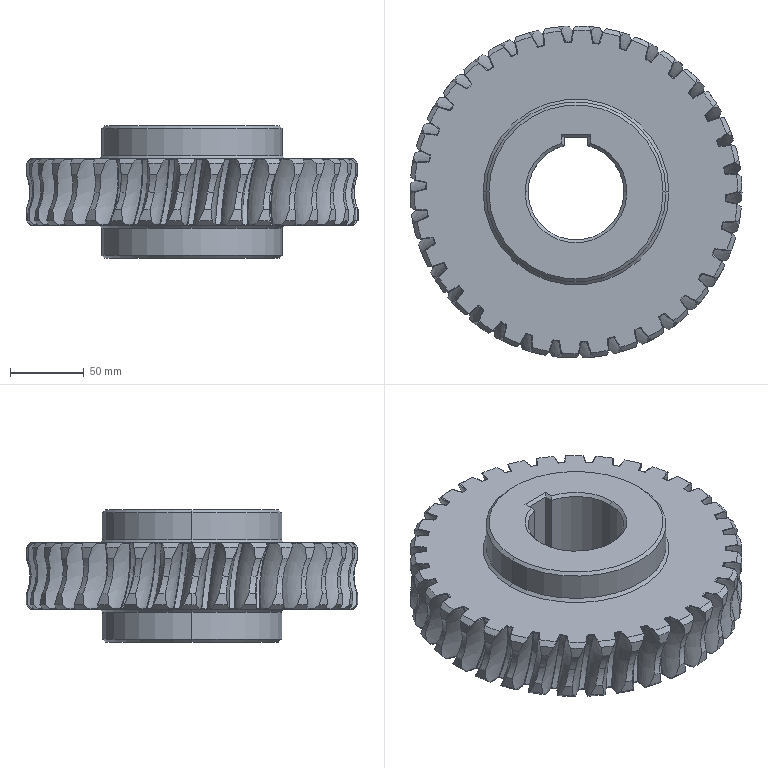Part | SolidWorks | features Chamfer 2, ICE 2, CirPattern 1, Extrusion 1, Fillet 1, Helix 1, MirrorPattern 1, RevCut 1, SweepCut 1 | 1 solid | 752 faces | box 225 x 225 x 90 mm | volume 1797406 mm3 | spline 510 | cone 84 | cylinder 76 | torus 69 | plane 13 | commonest cylinder face diameters 225 x69 122 x4 65 x3